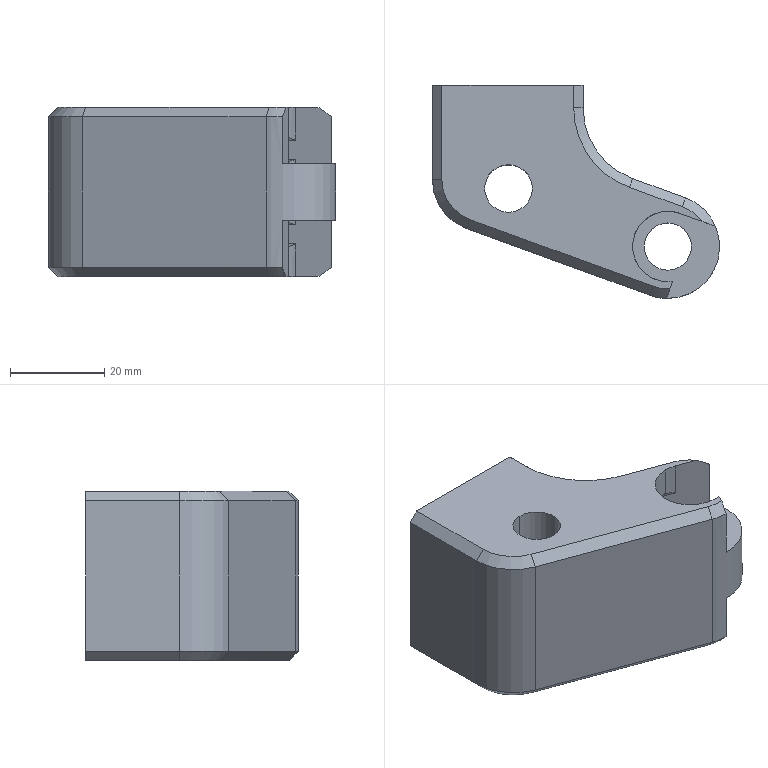Part | NX | features BREP 1 | 1 solid | 69 faces | box 61 x 45.195 x 36 mm | volume 49071 mm3 | cylinder 30 | plane 30 | cone 9 | commonest cylinder face diameters 15 x9 2 x8 4.06 x4 8.4 x2 10.04 x2 10.1 x2